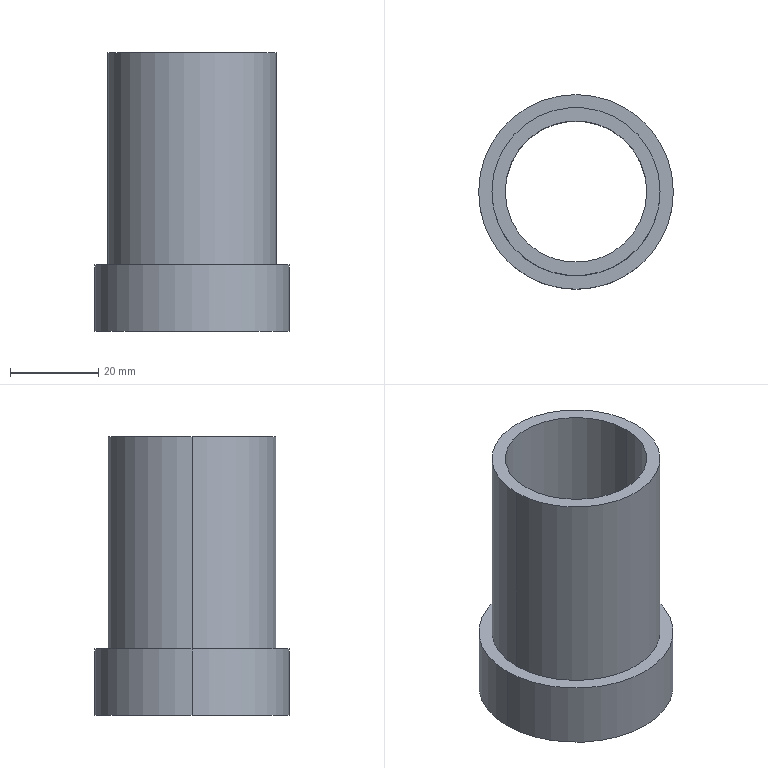Part | SolidWorks | features Extrusion 1, ICE 1 | 1 solid | 9 faces | box 44 x 44 x 63 mm | volume 26578 mm3 | cylinder 6 | plane 3 | commonest cylinder face diameters 32 x2 38 x2 44 x2
STEP:
#1=CARTESIAN_POINT('',(19.,0.,63.));
#2=VERTEX_POINT('',#1);
#3=CARTESIAN_POINT('',(-19.,0.,63.));
#4=VERTEX_POINT('',#3);
#5=CARTESIAN_POINT('',(0.,0.,63.));
#6=DIRECTION('',(0.,0.,1.));
#7=DIRECTION('',(1.,0.,0.));
#8=AXIS2_PLACEMENT_3D('',#5,#6,#7);
#9=CIRCLE('',#8,19.);
#10=EDGE_CURVE('',#2,#4,#9,.T.);
#11=ORIENTED_EDGE('',*,*,#10,.F.);
#12=CARTESIAN_POINT('',(19.,0.,15.));
#13=VERTEX_POINT('',#12);
#14=CARTESIAN_POINT('',(19.,0.,63.));
#15=DIRECTION('',(0.,0.,-1.));
#16=VECTOR('',#15,1000.);
#17=LINE('',#14,#16);
#18=EDGE_CURVE('',#2,#13,#17,.T.);
#19=ORIENTED_EDGE('',*,*,#18,.T.);
#20=CARTESIAN_POINT('',(-19.,0.,15.));
#21=VERTEX_POINT('',#20);
#22=CARTESIAN_POINT('',(0.,0.,15.));
#23=DIRECTION('',(0.,0.,1.));
#24=DIRECTION('',(1.,0.,0.));
#25=AXIS2_PLACEMENT_3D('',#22,#23,#24);
#26=CIRCLE('',#25,19.);
#27=EDGE_CURVE('',#13,#21,#26,.T.);
#28=ORIENTED_EDGE('',*,*,#27,.T.);
#29=CARTESIAN_POINT('',(-19.,0.,63.));
#30=DIRECTION('',(0.,0.,-1.));
#31=VECTOR('',#30,1000.);
#32=LINE('',#29,#31);
#33=EDGE_CURVE('',#4,#21,#32,.T.);
#34=ORIENTED_EDGE('',*,*,#33,.F.);
#35=EDGE_LOOP('',(#11,#19,#28,#34));
#36=FACE_OUTER_BOUND('',#35,.T.);
#37=CARTESIAN_POINT('',(0.,0.,63.));
#38=DIRECTION('',(0.,0.,-1.));
#39=DIRECTION('',(-1.,0.,0.));
#40=AXIS2_PLACEMENT_3D('',#37,#38,#39);
#41=CYLINDRICAL_SURFACE('',#40,19.);
#42=ADVANCED_FACE('',(#36),#41,.T.);
#43=CARTESIAN_POINT('',(-16.,0.,63.));
#44=VERTEX_POINT('',#43);
#45=CARTESIAN_POINT('',(16.,0.,63.));
#46=VERTEX_POINT('',#45);
#47=CARTESIAN_POINT('',(0.,0.,63.));
#48=DIRECTION('',(0.,0.,1.));
#49=DIRECTION('',(1.,0.,0.));
#50=AXIS2_PLACEMENT_3D('',#47,#48,#49);
#51=CIRCLE('',#50,16.);
#52=EDGE_CURVE('',#44,#46,#51,.T.);
#53=ORIENTED_EDGE('',*,*,#52,.T.);
#54=CARTESIAN_POINT('',(16.,0.,0.));
#55=VERTEX_POINT('',#54);
#56=CARTESIAN_POINT('',(16.,0.,15.));
#57=DIRECTION('',(0.,0.,-1.));
#58=VECTOR('',#57,1000.);
#59=LINE('',#56,#58);
#60=EDGE_CURVE('',#46,#55,#59,.T.);
#61=ORIENTED_EDGE('',*,*,#60,.T.);
#62=CARTESIAN_POINT('',(-16.,0.,0.));
#63=VERTEX_POINT('',#62);
#64=CARTESIAN_POINT('',(0.,0.,0.));
#65=DIRECTION('',(0.,0.,1.));
#66=DIRECTION('',(1.,0.,0.));
#67=AXIS2_PLACEMENT_3D('',#64,#65,#66);
#68=CIRCLE('',#67,16.);
#69=EDGE_CURVE('',#63,#55,#68,.T.);
#70=ORIENTED_EDGE('',*,*,#69,.F.);
#71=CARTESIAN_POINT('',(-16.,0.,15.));
#72=DIRECTION('',(0.,0.,-1.));
#73=VECTOR('',#72,1000.);
#74=LINE('',#71,#73);
#75=EDGE_CURVE('',#44,#63,#74,.T.);
#76=ORIENTED_EDGE('',*,*,#75,.F.);
#77=EDGE_LOOP('',(#53,#61,#70,#76));
#78=FACE_OUTER_BOUND('',#77,.T.);
#79=CARTESIAN_POINT('',(0.,0.,15.));
#80=DIRECTION('',(0.,0.,-1.));
#81=DIRECTION('',(-1.,0.,0.));
#82=AXIS2_PLACEMENT_3D('',#79,#80,#81);
#83=CYLINDRICAL_SURFACE('',#82,16.);
#84=ADVANCED_FACE('',(#78),#83,.F.);
#85=CARTESIAN_POINT('',(22.,0.,15.));
#86=VERTEX_POINT('',#85);
#87=CARTESIAN_POINT('',(-22.,0.,15.));
#88=VERTEX_POINT('',#87);
#89=CARTESIAN_POINT('',(0.,0.,15.));
#90=DIRECTION('',(0.,0.,1.));
#91=DIRECTION('',(1.,0.,0.));
#92=AXIS2_PLACEMENT_3D('',#89,#90,#91);
#93=CIRCLE('',#92,22.);
#94=EDGE_CURVE('',#86,#88,#93,.T.);
#95=ORIENTED_EDGE('',*,*,#94,.F.);
#96=CARTESIAN_POINT('',(22.,0.,0.));
#97=VERTEX_POINT('',#96);
#98=CARTESIAN_POINT('',(22.,0.,15.));
#99=DIRECTION('',(0.,0.,-1.));
#100=VECTOR('',#99,1000.);
#101=LINE('',#98,#100);
#102=EDGE_CURVE('',#86,#97,#101,.T.);
#103=ORIENTED_EDGE('',*,*,#102,.T.);
#104=CARTESIAN_POINT('',(-22.,0.,0.));
#105=VERTEX_POINT('',#104);
#106=CARTESIAN_POINT('',(0.,0.,0.));
#107=DIRECTION('',(0.,0.,1.));
#108=DIRECTION('',(1.,0.,0.));
#109=AXIS2_PLACEMENT_3D('',#106,#107,#108);
#110=CIRCLE('',#109,22.);
#111=EDGE_CURVE('',#97,#105,#110,.T.);
#112=ORIENTED_EDGE('',*,*,#111,.T.);
#113=CARTESIAN_POINT('',(-22.,0.,15.));
#114=DIRECTION('',(0.,0.,-1.));
#115=VECTOR('',#114,1000.);
#116=LINE('',#113,#115);
#117=EDGE_CURVE('',#88,#105,#116,.T.);
#118=ORIENTED_EDGE('',*,*,#117,.F.);
#119=EDGE_LOOP('',(#95,#103,#112,#118));
#120=FACE_OUTER_BOUND('',#119,.T.);
#121=CARTESIAN_POINT('',(0.,0.,15.));
#122=DIRECTION('',(0.,0.,-1.));
#123=DIRECTION('',(-1.,0.,0.));
#124=AXIS2_PLACEMENT_3D('',#121,#122,#123);
#125=CYLINDRICAL_SURFACE('',#124,22.);
#126=ADVANCED_FACE('',(#120),#125,.T.);
#127=CARTESIAN_POINT('',(0.,0.,15.));
#128=DIRECTION('',(0.,0.,1.));
#129=DIRECTION('',(1.,0.,0.));
#130=AXIS2_PLACEMENT_3D('',#127,#128,#129);
#131=CIRCLE('',#130,22.);
#132=EDGE_CURVE('',#88,#86,#131,.T.);
#133=ORIENTED_EDGE('',*,*,#132,.T.);
#134=ORIENTED_EDGE('',*,*,#94,.T.);
#135=EDGE_LOOP('',(#133,#134));
#136=FACE_OUTER_BOUND('',#135,.T.);
#137=CARTESIAN_POINT('',(0.,0.,15.));
#138=DIRECTION('',(0.,0.,1.));
#139=DIRECTION('',(1.,0.,0.));
#140=AXIS2_PLACEMENT_3D('',#137,#138,#139);
#141=CIRCLE('',#140,19.);
#142=EDGE_CURVE('',#21,#13,#141,.T.);
#143=ORIENTED_EDGE('',*,*,#142,.F.);
#144=ORIENTED_EDGE('',*,*,#27,.F.);
#145=EDGE_LOOP('',(#143,#144));
#146=FACE_BOUND('',#145,.T.);
#147=CARTESIAN_POINT('',(0.,0.,15.));
#148=DIRECTION('',(0.,0.,1.));
#149=DIRECTION('',(1.,0.,0.));
#150=AXIS2_PLACEMENT_3D('',#147,#148,#149);
#151=PLANE('',#150);
#152=ADVANCED_FACE('',(#136,#146),#151,.T.);
#153=CARTESIAN_POINT('',(0.,0.,0.));
#154=DIRECTION('',(0.,0.,1.));
#155=DIRECTION('',(1.,0.,0.));
#156=AXIS2_PLACEMENT_3D('',#153,#154,#155);
#157=CIRCLE('',#156,22.);
#158=EDGE_CURVE('',#105,#97,#157,.T.);
#159=ORIENTED_EDGE('',*,*,#158,.F.);
#160=ORIENTED_EDGE('',*,*,#111,.F.);
#161=EDGE_LOOP('',(#159,#160));
#162=FACE_OUTER_BOUND('',#161,.T.);
#163=ORIENTED_EDGE('',*,*,#69,.T.);
#164=CARTESIAN_POINT('',(0.,0.,0.));
#165=DIRECTION('',(0.,0.,1.));
#166=DIRECTION('',(1.,0.,0.));
#167=AXIS2_PLACEMENT_3D('',#164,#165,#166);
#168=CIRCLE('',#167,16.);
#169=EDGE_CURVE('',#55,#63,#168,.T.);
#170=ORIENTED_EDGE('',*,*,#169,.T.);
#171=EDGE_LOOP('',(#163,#170));
#172=FACE_BOUND('',#171,.T.);
#173=CARTESIAN_POINT('',(0.,0.,0.));
#174=DIRECTION('',(0.,0.,1.));
#175=DIRECTION('',(1.,0.,0.));
#176=AXIS2_PLACEMENT_3D('',#173,#174,#175);
#177=PLANE('',#176);
#178=ADVANCED_FACE('',(#162,#172),#177,.F.);
#179=ORIENTED_EDGE('',*,*,#102,.F.);
#180=ORIENTED_EDGE('',*,*,#132,.F.);
#181=ORIENTED_EDGE('',*,*,#117,.T.);
#182=ORIENTED_EDGE('',*,*,#158,.T.);
#183=EDGE_LOOP('',(#179,#180,#181,#182));
#184=FACE_OUTER_BOUND('',#183,.T.);
#185=CARTESIAN_POINT('',(0.,0.,15.));
#186=DIRECTION('',(0.,0.,-1.));
#187=DIRECTION('',(-1.,0.,0.));
#188=AXIS2_PLACEMENT_3D('',#185,#186,#187);
#189=CYLINDRICAL_SURFACE('',#188,22.);
#190=ADVANCED_FACE('',(#184),#189,.T.);
#191=ORIENTED_EDGE('',*,*,#60,.F.);
#192=CARTESIAN_POINT('',(0.,0.,63.));
#193=DIRECTION('',(0.,0.,1.));
#194=DIRECTION('',(1.,0.,0.));
#195=AXIS2_PLACEMENT_3D('',#192,#193,#194);
#196=CIRCLE('',#195,16.);
#197=EDGE_CURVE('',#46,#44,#196,.T.);
#198=ORIENTED_EDGE('',*,*,#197,.T.);
#199=ORIENTED_EDGE('',*,*,#75,.T.);
#200=ORIENTED_EDGE('',*,*,#169,.F.);
#201=EDGE_LOOP('',(#191,#198,#199,#200));
#202=FACE_OUTER_BOUND('',#201,.T.);
#203=CARTESIAN_POINT('',(0.,0.,15.));
#204=DIRECTION('',(0.,0.,-1.));
#205=DIRECTION('',(-1.,0.,0.));
#206=AXIS2_PLACEMENT_3D('',#203,#204,#205);
#207=CYLINDRICAL_SURFACE('',#206,16.);
#208=ADVANCED_FACE('',(#202),#207,.F.);
#209=CARTESIAN_POINT('',(0.,0.,63.));
#210=DIRECTION('',(0.,0.,1.));
#211=DIRECTION('',(1.,0.,0.));
#212=AXIS2_PLACEMENT_3D('',#209,#210,#211);
#213=CIRCLE('',#212,19.);
#214=EDGE_CURVE('',#4,#2,#213,.T.);
#215=ORIENTED_EDGE('',*,*,#214,.T.);
#216=ORIENTED_EDGE('',*,*,#10,.T.);
#217=EDGE_LOOP('',(#215,#216));
#218=FACE_OUTER_BOUND('',#217,.T.);
#219=ORIENTED_EDGE('',*,*,#52,.F.);
#220=ORIENTED_EDGE('',*,*,#197,.F.);
#221=EDGE_LOOP('',(#219,#220));
#222=FACE_BOUND('',#221,.T.);
#223=CARTESIAN_POINT('',(0.,0.,63.));
#224=DIRECTION('',(0.,0.,1.));
#225=DIRECTION('',(1.,0.,0.));
#226=AXIS2_PLACEMENT_3D('',#223,#224,#225);
#227=PLANE('',#226);
#228=ADVANCED_FACE('',(#218,#222),#227,.T.);
#229=ORIENTED_EDGE('',*,*,#18,.F.);
#230=ORIENTED_EDGE('',*,*,#214,.F.);
#231=ORIENTED_EDGE('',*,*,#33,.T.);
#232=ORIENTED_EDGE('',*,*,#142,.T.);
#233=EDGE_LOOP('',(#229,#230,#231,#232));
#234=FACE_OUTER_BOUND('',#233,.T.);
#235=CARTESIAN_POINT('',(0.,0.,63.));
#236=DIRECTION('',(0.,0.,-1.));
#237=DIRECTION('',(-1.,0.,0.));
#238=AXIS2_PLACEMENT_3D('',#235,#236,#237);
#239=CYLINDRICAL_SURFACE('',#238,19.);
#240=ADVANCED_FACE('',(#234),#239,.T.);
#241=CLOSED_SHELL('',(#42,#84,#126,#152,#178,#190,#208,#228,#240));
#242=MANIFOLD_SOLID_BREP('',#241);
#243=CARTESIAN_POINT('',(0.,0.,0.));
#244=DIRECTION('',(0.,0.,1.));
#245=DIRECTION('',(1.,0.,0.));
#246=AXIS2_PLACEMENT_3D('',#243,#244,#245);
#247=(LENGTH_UNIT()NAMED_UNIT(*)SI_UNIT(.MILLI.,.METRE.));
#248=UNCERTAINTY_MEASURE_WITH_UNIT(LENGTH_MEASURE(0.00001),#247,'','');
#249=(NAMED_UNIT(*)PLANE_ANGLE_UNIT()SI_UNIT($,.RADIAN.));
#250=(NAMED_UNIT(*)SI_UNIT($,.STERADIAN.)SOLID_ANGLE_UNIT());
#251=(GEOMETRIC_REPRESENTATION_CONTEXT(3)GLOBAL_UNCERTAINTY_ASSIGNED_CONTEXT((#248))GLOBAL_UNIT_ASSIGNED_CONTEXT((#247,#249,#250))REPRESENTATION_CONTEXT('',''));
#252=ADVANCED_BREP_SHAPE_REPRESENTATION('',(#242,#246),#251);